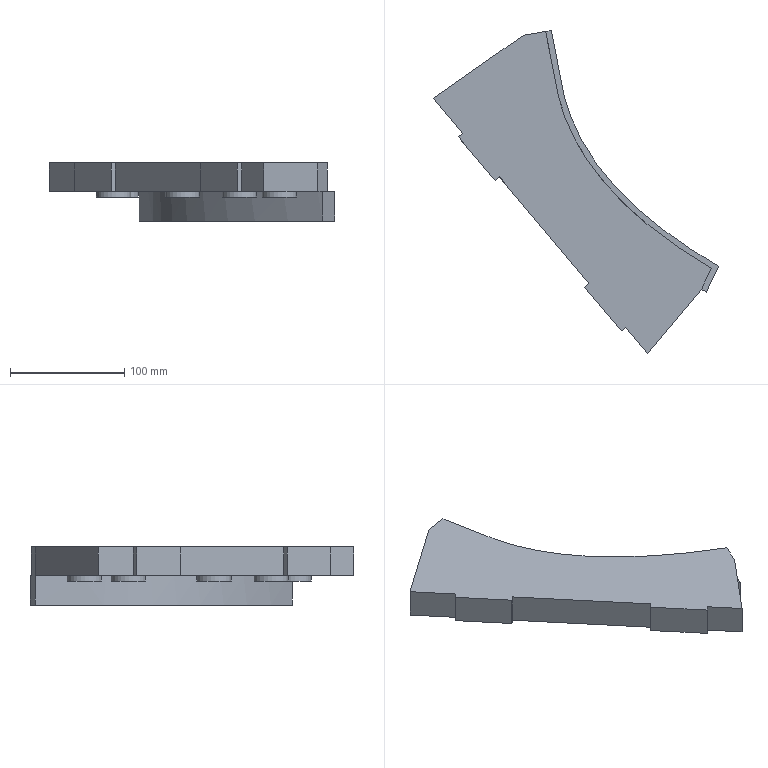Part | NX | features solid 2 | 1 solid | 31 faces | box 249.689 x 282.861 x 51 mm | volume 776005 mm3 | plane 23 | cylinder 5 | spline 3 | commonest cylinder face diameters 30 x5
STEP:
#1=CARTESIAN_POINT('',(-785.62,49.22,20.));
#2=VERTEX_POINT('',#1);
#3=CARTESIAN_POINT('',(-640.688,-158.312,20.));
#4=VERTEX_POINT('',#3);
#5=CARTESIAN_POINT('',(-785.62,49.22,20.));
#6=CARTESIAN_POINT('',(-784.592,43.889,20.));
#7=CARTESIAN_POINT('',(-782.539,33.228,20.));
#8=CARTESIAN_POINT('',(-779.967,19.892,20.));
#9=CARTESIAN_POINT('',(-777.921,9.245,20.));
#10=CARTESIAN_POINT('',(-776.403,1.242,20.));
#11=CARTESIAN_POINT('',(-774.716,-6.95,20.));
#12=CARTESIAN_POINT('',(-771.799,-17.805,20.));
#13=CARTESIAN_POINT('',(-767.13,-31.015,20.));
#14=CARTESIAN_POINT('',(-757.579,-51.275,20.));
#15=CARTESIAN_POINT('',(-742.261,-74.623,20.));
#16=CARTESIAN_POINT('',(-720.074,-99.485,20.));
#17=CARTESIAN_POINT('',(-687.034,-128.8,20.));
#18=CARTESIAN_POINT('',(-659.634,-147.246,20.));
#19=CARTESIAN_POINT('',(-640.688,-158.312,20.));
#20=B_SPLINE_CURVE_WITH_KNOTS('',3,(#5,#6,#7,#8,#9,#10,#11,#12,#13,#14,#15,#16,#17,#18,#19),.UNSPECIFIED.,.F.,.F.,(4,1,1,1,1,1,1,1,1,1,1,1,4),(-0.0002983,0.06115,0.1226,0.1533,0.184,0.2148,0.2455,0.3069,0.3684,0.4913,0.6141,0.737,0.9828),.UNSPECIFIED.);
#21=EDGE_CURVE('',#2,#4,#20,.T.);
#22=ORIENTED_EDGE('',*,*,#21,.T.);
#23=CARTESIAN_POINT('',(-649.178,-176.519,20.));
#24=VERTEX_POINT('',#23);
#25=CARTESIAN_POINT('',(-638.752,-154.162,20.));
#26=DIRECTION('',(-0.4226,-0.9063,0.));
#27=VECTOR('',#26,1000.);
#28=LINE('',#25,#27);
#29=EDGE_CURVE('',#4,#24,#28,.T.);
#30=ORIENTED_EDGE('',*,*,#29,.T.);
#31=CARTESIAN_POINT('',(-644.823,-179.011,20.));
#32=VERTEX_POINT('',#31);
#33=CARTESIAN_POINT('',(-805.318,45.747,20.));
#34=CARTESIAN_POINT('',(-803.55,36.568,20.));
#35=CARTESIAN_POINT('',(-801.348,25.134,20.));
#36=CARTESIAN_POINT('',(-798.703,11.417,20.));
#37=CARTESIAN_POINT('',(-797.422,4.72,20.));
#38=CARTESIAN_POINT('',(-796.1,-2.196,20.));
#39=CARTESIAN_POINT('',(-794.091,-12.171,20.));
#40=CARTESIAN_POINT('',(-790.472,-25.289,20.));
#41=CARTESIAN_POINT('',(-782.995,-45.31,20.));
#42=CARTESIAN_POINT('',(-770.656,-68.68,20.));
#43=CARTESIAN_POINT('',(-752.344,-93.703,20.));
#44=CARTESIAN_POINT('',(-731.663,-115.921,20.));
#45=CARTESIAN_POINT('',(-709.317,-135.702,20.));
#46=CARTESIAN_POINT('',(-680.689,-157.352,20.));
#47=CARTESIAN_POINT('',(-658.817,-171.096,20.));
#48=CARTESIAN_POINT('',(-644.823,-179.011,20.));
#49=B_SPLINE_CURVE_WITH_KNOTS('',3,(#33,#34,#35,#36,#37,#38,#39,#40,#41,#42,#43,#44,#45,#46,#47,#48),.UNSPECIFIED.,.F.,.F.,(4,1,1,1,1,1,1,1,1,1,1,1,1,4),(0.,0.1048,0.1307,0.1565,0.1824,0.2082,0.2599,0.3116,0.4149,0.5183,0.6217,0.725,0.8284,1.),.UNSPECIFIED.);
#50=EDGE_CURVE('',#32,#24,#49,.F.);
#51=ORIENTED_EDGE('',*,*,#50,.F.);
#52=CARTESIAN_POINT('',(-634.221,-156.275,20.));
#53=VERTEX_POINT('',#52);
#54=CARTESIAN_POINT('',(-634.221,-156.275,20.));
#55=DIRECTION('',(0.4226,0.9063,0.));
#56=VECTOR('',#55,1000.);
#57=LINE('',#54,#56);
#58=EDGE_CURVE('',#32,#53,#57,.T.);
#59=ORIENTED_EDGE('',*,*,#58,.T.);
#60=CARTESIAN_POINT('',(-780.695,50.088,20.));
#61=VERTEX_POINT('',#60);
#62=CARTESIAN_POINT('',(-780.695,50.088,20.));
#63=CARTESIAN_POINT('',(-778.803,40.269,20.));
#64=CARTESIAN_POINT('',(-776.28,27.176,20.));
#65=CARTESIAN_POINT('',(-773.127,10.811,20.));
#66=CARTESIAN_POINT('',(-771.556,2.503,20.));
#67=CARTESIAN_POINT('',(-770.053,-4.764,20.));
#68=CARTESIAN_POINT('',(-768.05,-12.691,20.));
#69=CARTESIAN_POINT('',(-763.621,-26.574,20.));
#70=CARTESIAN_POINT('',(-751.782,-52.713,20.));
#71=CARTESIAN_POINT('',(-727.402,-85.879,20.));
#72=CARTESIAN_POINT('',(-691.163,-119.147,20.));
#73=CARTESIAN_POINT('',(-659.144,-141.522,20.));
#74=CARTESIAN_POINT('',(-639.695,-153.145,20.));
#75=CARTESIAN_POINT('',(-634.221,-156.275,20.));
#76=B_SPLINE_CURVE_WITH_KNOTS('',3,(#62,#63,#64,#65,#66,#67,#68,#69,#70,#71,#72,#73,#74,#75),.UNSPECIFIED.,.F.,.F.,(4,1,1,1,1,1,1,1,1,1,1,4),(0.,0.1132,0.1509,0.1886,0.2088,0.2349,0.2811,0.3736,0.5586,0.7436,0.9286,1.),.UNSPECIFIED.);
#77=EDGE_CURVE('',#53,#61,#76,.F.);
#78=ORIENTED_EDGE('',*,*,#77,.T.);
#79=CARTESIAN_POINT('',(-780.695,50.088,20.));
#80=DIRECTION('',(0.9848,0.1736,0.));
#81=VECTOR('',#80,1000.);
#82=LINE('',#79,#81);
#83=EDGE_CURVE('',#2,#61,#82,.T.);
#84=ORIENTED_EDGE('',*,*,#83,.F.);
#85=EDGE_LOOP('',(#22,#30,#51,#59,#78,#84));
#86=FACE_BOUND('',#85,.T.);
#87=CARTESIAN_POINT('',(-565.659,-207.42,20.));
#88=DIRECTION('',(0.,0.,1.));
#89=DIRECTION('',(1.,0.,0.));
#90=AXIS2_PLACEMENT_3D('',#87,#88,#89);
#91=PLANE('',#90);
#92=ADVANCED_FACE('',(#86),#91,.T.);
#93=CARTESIAN_POINT('',(-669.708,-173.137,15.));
#94=VERTEX_POINT('',#93);
#95=CARTESIAN_POINT('',(-682.698,-180.637,15.));
#96=DIRECTION('',(0.,0.,-1.));
#97=DIRECTION('',(0.866,0.5,0.));
#98=AXIS2_PLACEMENT_3D('',#95,#96,#97);
#99=CIRCLE('',#98,15.);
#100=EDGE_CURVE('',#94,#94,#99,.T.);
#101=ORIENTED_EDGE('',*,*,#100,.T.);
#102=EDGE_LOOP('',(#101));
#103=FACE_BOUND('',#102,.T.);
#104=CARTESIAN_POINT('',(-682.698,-180.637,15.));
#105=DIRECTION('',(0.,0.,-1.));
#106=DIRECTION('',(-0.866,-0.5,0.));
#107=AXIS2_PLACEMENT_3D('',#104,#105,#106);
#108=PLANE('',#107);
#109=ADVANCED_FACE('',(#103),#108,.T.);
#110=ORIENTED_EDGE('',*,*,#100,.F.);
#111=EDGE_LOOP('',(#110));
#112=FACE_BOUND('',#111,.T.);
#113=CARTESIAN_POINT('',(-669.708,-173.137,20.));
#114=VERTEX_POINT('',#113);
#115=CARTESIAN_POINT('',(-682.698,-180.637,20.));
#116=DIRECTION('',(0.,0.,-1.));
#117=DIRECTION('',(0.866,0.5,0.));
#118=AXIS2_PLACEMENT_3D('',#115,#116,#117);
#119=CIRCLE('',#118,15.);
#120=EDGE_CURVE('',#114,#114,#119,.T.);
#121=ORIENTED_EDGE('',*,*,#120,.T.);
#122=EDGE_LOOP('',(#121));
#123=FACE_BOUND('',#122,.T.);
#124=CARTESIAN_POINT('',(-682.698,-180.637,20.));
#125=DIRECTION('',(0.,0.,-1.));
#126=DIRECTION('',(-0.866,-0.5,0.));
#127=AXIS2_PLACEMENT_3D('',#124,#125,#126);
#128=CYLINDRICAL_SURFACE('',#127,15.);
#129=ADVANCED_FACE('',(#112,#123),#128,.T.);
#130=CARTESIAN_POINT('',(-805.318,45.747,20.));
#131=VERTEX_POINT('',#130);
#132=CARTESIAN_POINT('',(-649.178,-176.519,20.));
#133=CARTESIAN_POINT('',(-659.441,-170.582,20.));
#134=CARTESIAN_POINT('',(-679.515,-158.013,20.));
#135=CARTESIAN_POINT('',(-708.226,-136.801,20.));
#136=CARTESIAN_POINT('',(-730.28,-117.148,20.));
#137=CARTESIAN_POINT('',(-746.505,-99.916,20.));
#138=CARTESIAN_POINT('',(-757.891,-86.111,20.));
#139=CARTESIAN_POINT('',(-768.135,-71.661,20.));
#140=CARTESIAN_POINT('',(-777.154,-56.472,20.));
#141=CARTESIAN_POINT('',(-784.851,-40.491,20.));
#142=CARTESIAN_POINT('',(-790.016,-26.444,20.));
#143=CARTESIAN_POINT('',(-793.291,-15.081,20.));
#144=CARTESIAN_POINT('',(-795.289,-6.451,20.));
#145=CARTESIAN_POINT('',(-796.948,2.251,20.));
#146=CARTESIAN_POINT('',(-799.169,13.852,20.));
#147=CARTESIAN_POINT('',(-801.968,28.349,20.));
#148=CARTESIAN_POINT('',(-804.201,39.947,20.));
#149=CARTESIAN_POINT('',(-805.318,45.747,20.));
#150=B_SPLINE_CURVE_WITH_KNOTS('',3,(#132,#133,#134,#135,#136,#137,#138,#139,#140,#141,#142,#143,#144,#145,#146,#147,#148,#149),.UNSPECIFIED.,.F.,.F.,(4,1,1,1,1,1,1,1,1,1,1,1,1,1,1,4),(0.1002,0.1358,0.1714,0.207,0.2248,0.2425,0.2603,0.2781,0.2959,0.3137,0.3226,0.3315,0.3404,0.3493,0.3671,0.3849),.UNSPECIFIED.);
#151=EDGE_CURVE('',#131,#24,#150,.F.);
#152=ORIENTED_EDGE('',*,*,#151,.F.);
#153=CARTESIAN_POINT('',(-805.318,45.747,-6.));
#154=VERTEX_POINT('',#153);
#155=CARTESIAN_POINT('',(-805.318,45.747,45.));
#156=DIRECTION('',(0.,0.,-1.));
#157=VECTOR('',#156,1000.);
#158=LINE('',#155,#157);
#159=EDGE_CURVE('',#131,#154,#158,.T.);
#160=ORIENTED_EDGE('',*,*,#159,.T.);
#161=CARTESIAN_POINT('',(-644.823,-179.011,-6.));
#162=VERTEX_POINT('',#161);
#163=CARTESIAN_POINT('',(-805.318,45.747,-6.));
#164=CARTESIAN_POINT('',(-803.55,36.568,-6.));
#165=CARTESIAN_POINT('',(-801.348,25.134,-6.));
#166=CARTESIAN_POINT('',(-798.703,11.417,-6.));
#167=CARTESIAN_POINT('',(-797.422,4.72,-6.));
#168=CARTESIAN_POINT('',(-796.1,-2.196,-6.));
#169=CARTESIAN_POINT('',(-794.091,-12.171,-6.));
#170=CARTESIAN_POINT('',(-790.472,-25.289,-6.));
#171=CARTESIAN_POINT('',(-782.995,-45.31,-6.));
#172=CARTESIAN_POINT('',(-770.656,-68.68,-6.));
#173=CARTESIAN_POINT('',(-752.344,-93.703,-6.));
#174=CARTESIAN_POINT('',(-731.663,-115.921,-6.));
#175=CARTESIAN_POINT('',(-709.317,-135.702,-6.));
#176=CARTESIAN_POINT('',(-680.689,-157.352,-6.));
#177=CARTESIAN_POINT('',(-658.817,-171.096,-6.));
#178=CARTESIAN_POINT('',(-644.823,-179.011,-6.));
#179=B_SPLINE_CURVE_WITH_KNOTS('',3,(#163,#164,#165,#166,#167,#168,#169,#170,#171,#172,#173,#174,#175,#176,#177,#178),.UNSPECIFIED.,.F.,.F.,(4,1,1,1,1,1,1,1,1,1,1,1,1,4),(0.,0.1048,0.1307,0.1565,0.1824,0.2082,0.2599,0.3116,0.4149,0.5183,0.6217,0.725,0.8284,1.),.UNSPECIFIED.);
#180=EDGE_CURVE('',#154,#162,#179,.T.);
#181=ORIENTED_EDGE('',*,*,#180,.T.);
#182=CARTESIAN_POINT('',(-644.823,-179.011,45.));
#183=DIRECTION('',(0.,0.,-1.));
#184=VECTOR('',#183,1000.);
#185=LINE('',#182,#184);
#186=EDGE_CURVE('',#32,#162,#185,.T.);
#187=ORIENTED_EDGE('',*,*,#186,.F.);
#188=ORIENTED_EDGE('',*,*,#50,.T.);
#189=EDGE_LOOP('',(#152,#160,#181,#187,#188));
#190=FACE_BOUND('',#189,.T.);
#191=CARTESIAN_POINT('',(-805.318,45.747,20.));
#192=CARTESIAN_POINT('',(-805.318,45.747,-6.));
#193=CARTESIAN_POINT('',(-804.264,40.275,20.));
#194=CARTESIAN_POINT('',(-804.264,40.275,-6.));
#195=CARTESIAN_POINT('',(-802.161,29.355,20.));
#196=CARTESIAN_POINT('',(-802.161,29.355,-6.));
#197=CARTESIAN_POINT('',(-799.507,15.599,20.));
#198=CARTESIAN_POINT('',(-799.507,15.599,-6.));
#199=CARTESIAN_POINT('',(-797.435,4.808,20.));
#200=CARTESIAN_POINT('',(-797.435,4.808,-6.));
#201=CARTESIAN_POINT('',(-795.845,-3.597,20.));
#202=CARTESIAN_POINT('',(-795.845,-3.597,-6.));
#203=CARTESIAN_POINT('',(-793.889,-12.805,20.));
#204=CARTESIAN_POINT('',(-793.889,-12.805,-6.));
#205=CARTESIAN_POINT('',(-790.396,-25.393,20.));
#206=CARTESIAN_POINT('',(-790.396,-25.393,-6.));
#207=CARTESIAN_POINT('',(-784.843,-40.631,20.));
#208=CARTESIAN_POINT('',(-784.843,-40.631,-6.));
#209=CARTESIAN_POINT('',(-776.44,-57.876,20.));
#210=CARTESIAN_POINT('',(-776.44,-57.876,-6.));
#211=CARTESIAN_POINT('',(-766.575,-74.079,20.));
#212=CARTESIAN_POINT('',(-766.575,-74.079,-6.));
#213=CARTESIAN_POINT('',(-751.833,-94.216,20.));
#214=CARTESIAN_POINT('',(-751.833,-94.216,-6.));
#215=CARTESIAN_POINT('',(-731.088,-116.783,20.));
#216=CARTESIAN_POINT('',(-731.088,-116.783,-6.));
#217=CARTESIAN_POINT('',(-703.818,-140.307,20.));
#218=CARTESIAN_POINT('',(-703.818,-140.307,-6.));
#219=CARTESIAN_POINT('',(-675.037,-161.006,20.));
#220=CARTESIAN_POINT('',(-675.037,-161.006,-6.));
#221=CARTESIAN_POINT('',(-655.017,-173.245,20.));
#222=CARTESIAN_POINT('',(-655.017,-173.245,-6.));
#223=CARTESIAN_POINT('',(-644.823,-179.011,20.));
#224=CARTESIAN_POINT('',(-644.823,-179.011,-6.));
#225=B_SPLINE_SURFACE_WITH_KNOTS('',3,1,((#191,#192),(#193,#194),(#195,#196),(#197,#198),(#199,#200),(#201,#202),(#203,#204),(#205,#206),(#207,#208),(#209,#210),(#211,#212),(#213,#214),(#215,#216),(#217,#218),(#219,#220),(#221,#222),(#223,#224)),.SURF_OF_LINEAR_EXTRUSION.,.F.,.F.,.F.,(4,1,1,1,1,1,1,1,1,1,1,1,1,1,4),(2,2),(0.,0.0625,0.125,0.1562,0.1875,0.2188,0.25,0.3125,0.375,0.4375,0.5,0.625,0.75,0.875,1.),(0.,1.),.UNSPECIFIED.);
#226=ADVANCED_FACE('',(#190),#225,.F.);
#227=CARTESIAN_POINT('',(-634.221,-156.275,-6.));
#228=VERTEX_POINT('',#227);
#229=CARTESIAN_POINT('',(-634.221,-156.275,-6.));
#230=DIRECTION('',(-0.4226,-0.9063,0.));
#231=VECTOR('',#230,1000.);
#232=LINE('',#229,#231);
#233=EDGE_CURVE('',#228,#162,#232,.T.);
#234=ORIENTED_EDGE('',*,*,#233,.F.);
#235=CARTESIAN_POINT('',(-634.221,-156.275,45.));
#236=DIRECTION('',(0.,0.,-1.));
#237=VECTOR('',#236,1000.);
#238=LINE('',#235,#237);
#239=EDGE_CURVE('',#53,#228,#238,.T.);
#240=ORIENTED_EDGE('',*,*,#239,.F.);
#241=ORIENTED_EDGE('',*,*,#58,.F.);
#242=ORIENTED_EDGE('',*,*,#186,.T.);
#243=EDGE_LOOP('',(#234,#240,#241,#242));
#244=FACE_BOUND('',#243,.T.);
#245=CARTESIAN_POINT('',(-644.823,-179.011,45.));
#246=DIRECTION('',(0.9063,-0.4226,0.));
#247=DIRECTION('',(0.4226,0.9063,0.));
#248=AXIS2_PLACEMENT_3D('',#245,#246,#247);
#249=PLANE('',#248);
#250=ADVANCED_FACE('',(#244),#249,.T.);
#251=CARTESIAN_POINT('',(-649.178,-176.519,45.));
#252=VERTEX_POINT('',#251);
#253=CARTESIAN_POINT('',(-649.178,-176.519,20.));
#254=DIRECTION('',(0.,0.,-1.));
#255=VECTOR('',#254,1000.);
#256=LINE('',#253,#255);
#257=EDGE_CURVE('',#252,#24,#256,.T.);
#258=ORIENTED_EDGE('',*,*,#257,.F.);
#259=CARTESIAN_POINT('',(-696.38,-232.773,45.));
#260=VERTEX_POINT('',#259);
#261=CARTESIAN_POINT('',(-649.96,-177.452,45.));
#262=DIRECTION('',(-0.6428,-0.766,0.));
#263=VECTOR('',#262,1000.);
#264=LINE('',#261,#263);
#265=EDGE_CURVE('',#252,#260,#264,.T.);
#266=ORIENTED_EDGE('',*,*,#265,.T.);
#267=CARTESIAN_POINT('',(-696.38,-232.773,20.));
#268=VERTEX_POINT('',#267);
#269=CARTESIAN_POINT('',(-696.38,-232.773,45.));
#270=DIRECTION('',(0.,0.,-1.));
#271=VECTOR('',#270,1000.);
#272=LINE('',#269,#271);
#273=EDGE_CURVE('',#260,#268,#272,.T.);
#274=ORIENTED_EDGE('',*,*,#273,.T.);
#275=CARTESIAN_POINT('',(-649.96,-177.452,20.));
#276=DIRECTION('',(-0.6428,-0.766,0.));
#277=VECTOR('',#276,1000.);
#278=LINE('',#275,#277);
#279=EDGE_CURVE('',#24,#268,#278,.T.);
#280=ORIENTED_EDGE('',*,*,#279,.F.);
#281=EDGE_LOOP('',(#258,#266,#274,#280));
#282=FACE_BOUND('',#281,.T.);
#283=CARTESIAN_POINT('',(-649.178,-176.519,20.));
#284=DIRECTION('',(-0.766,0.6428,0.));
#285=DIRECTION('',(-0.6428,-0.766,0.));
#286=AXIS2_PLACEMENT_3D('',#283,#284,#285);
#287=PLANE('',#286);
#288=ADVANCED_FACE('',(#282),#287,.F.);
#289=ORIENTED_EDGE('',*,*,#29,.F.);
#290=CARTESIAN_POINT('',(-640.688,-158.312,45.));
#291=VERTEX_POINT('',#290);
#292=CARTESIAN_POINT('',(-640.688,-158.312,32.5));
#293=DIRECTION('',(0.,0.,1.));
#294=VECTOR('',#293,1000.);
#295=LINE('',#292,#294);
#296=EDGE_CURVE('',#291,#4,#295,.F.);
#297=ORIENTED_EDGE('',*,*,#296,.F.);
#298=CARTESIAN_POINT('',(-634.625,-145.31,45.));
#299=DIRECTION('',(-0.4226,-0.9063,0.));
#300=VECTOR('',#299,1000.);
#301=LINE('',#298,#300);
#302=EDGE_CURVE('',#291,#252,#301,.T.);
#303=ORIENTED_EDGE('',*,*,#302,.T.);
#304=ORIENTED_EDGE('',*,*,#257,.T.);
#305=EDGE_LOOP('',(#289,#297,#303,#304));
#306=FACE_BOUND('',#305,.T.);
#307=CARTESIAN_POINT('',(-638.752,-154.162,20.));
#308=DIRECTION('',(-0.9063,0.4226,0.));
#309=DIRECTION('',(-0.4226,-0.9063,0.));
#310=AXIS2_PLACEMENT_3D('',#307,#308,#309);
#311=PLANE('',#310);
#312=ADVANCED_FACE('',(#306),#311,.F.);
#313=CARTESIAN_POINT('',(-715.664,-209.791,45.));
#314=VERTEX_POINT('',#313);
#315=CARTESIAN_POINT('',(-715.664,-209.791,20.));
#316=VERTEX_POINT('',#315);
#317=CARTESIAN_POINT('',(-715.664,-209.791,45.));
#318=DIRECTION('',(0.,0.,-1.));
#319=VECTOR('',#318,1000.);
#320=LINE('',#317,#319);
#321=EDGE_CURVE('',#314,#316,#320,.T.);
#322=ORIENTED_EDGE('',*,*,#321,.F.);
#323=CARTESIAN_POINT('',(-719.494,-213.005,45.));
#324=VERTEX_POINT('',#323);
#325=CARTESIAN_POINT('',(-719.494,-213.005,45.));
#326=DIRECTION('',(0.766,0.6428,0.));
#327=VECTOR('',#326,1000.);
#328=LINE('',#325,#327);
#329=EDGE_CURVE('',#324,#314,#328,.T.);
#330=ORIENTED_EDGE('',*,*,#329,.F.);
#331=CARTESIAN_POINT('',(-719.494,-213.005,20.));
#332=VERTEX_POINT('',#331);
#333=CARTESIAN_POINT('',(-719.494,-213.005,45.));
#334=DIRECTION('',(0.,0.,-1.));
#335=VECTOR('',#334,1000.);
#336=LINE('',#333,#335);
#337=EDGE_CURVE('',#324,#332,#336,.T.);
#338=ORIENTED_EDGE('',*,*,#337,.T.);
#339=CARTESIAN_POINT('',(-719.494,-213.005,20.));
#340=DIRECTION('',(0.766,0.6428,0.));
#341=VECTOR('',#340,1000.);
#342=LINE('',#339,#341);
#343=EDGE_CURVE('',#332,#316,#342,.T.);
#344=ORIENTED_EDGE('',*,*,#343,.T.);
#345=EDGE_LOOP('',(#322,#330,#338,#344));
#346=FACE_BOUND('',#345,.T.);
#347=CARTESIAN_POINT('',(-719.494,-213.005,45.));
#348=DIRECTION('',(0.6428,-0.766,0.));
#349=DIRECTION('',(0.766,0.6428,0.));
#350=AXIS2_PLACEMENT_3D('',#347,#348,#349);
#351=PLANE('',#350);
#352=ADVANCED_FACE('',(#346),#351,.T.);
#353=ORIENTED_EDGE('',*,*,#321,.T.);
#354=CARTESIAN_POINT('',(-676.357,-256.636,20.));
#355=DIRECTION('',(-0.6428,0.766,0.));
#356=VECTOR('',#355,1000.);
#357=LINE('',#354,#356);
#358=EDGE_CURVE('',#268,#316,#357,.T.);
#359=ORIENTED_EDGE('',*,*,#358,.F.);
#360=ORIENTED_EDGE('',*,*,#273,.F.);
#361=CARTESIAN_POINT('',(-676.357,-256.636,45.));
#362=DIRECTION('',(-0.6428,0.766,0.));
#363=VECTOR('',#362,1000.);
#364=LINE('',#361,#363);
#365=EDGE_CURVE('',#260,#314,#364,.T.);
#366=ORIENTED_EDGE('',*,*,#365,.T.);
#367=EDGE_LOOP('',(#353,#359,#360,#366));
#368=FACE_BOUND('',#367,.T.);
#369=CARTESIAN_POINT('',(-676.357,-256.636,45.));
#370=DIRECTION('',(-0.766,-0.6428,0.));
#371=DIRECTION('',(0.6428,-0.766,0.));
#372=AXIS2_PLACEMENT_3D('',#369,#370,#371);
#373=PLANE('',#372);
#374=ADVANCED_FACE('',(#368),#373,.T.);
#375=CARTESIAN_POINT('',(-862.028,-43.139,45.));
#376=VERTEX_POINT('',#375);
#377=CARTESIAN_POINT('',(-858.198,-39.926,45.));
#378=VERTEX_POINT('',#377);
#379=CARTESIAN_POINT('',(-1200.954,-327.532,45.));
#380=DIRECTION('',(0.766,0.6428,0.));
#381=VECTOR('',#380,1000.);
#382=LINE('',#379,#381);
#383=EDGE_CURVE('',#376,#378,#382,.T.);
#384=ORIENTED_EDGE('',*,*,#383,.F.);
#385=CARTESIAN_POINT('',(-829.889,-81.442,45.));
#386=VERTEX_POINT('',#385);
#387=CARTESIAN_POINT('',(-816.294,-97.644,45.));
#388=DIRECTION('',(-0.6428,0.766,0.));
#389=VECTOR('',#388,1000.);
#390=LINE('',#387,#389);
#391=EDGE_CURVE('',#386,#376,#390,.T.);
#392=ORIENTED_EDGE('',*,*,#391,.F.);
#393=CARTESIAN_POINT('',(-826.059,-78.228,45.));
#394=VERTEX_POINT('',#393);
#395=CARTESIAN_POINT('',(-1168.815,-365.834,45.));
#396=DIRECTION('',(0.766,0.6428,0.));
#397=VECTOR('',#396,1000.);
#398=LINE('',#395,#397);
#399=EDGE_CURVE('',#386,#394,#398,.T.);
#400=ORIENTED_EDGE('',*,*,#399,.T.);
#401=CARTESIAN_POINT('',(-747.803,-171.489,45.));
#402=VERTEX_POINT('',#401);
#403=CARTESIAN_POINT('',(-676.357,-256.636,45.));
#404=DIRECTION('',(-0.6428,0.766,0.));
#405=VECTOR('',#404,1000.);
#406=LINE('',#403,#405);
#407=EDGE_CURVE('',#402,#394,#406,.T.);
#408=ORIENTED_EDGE('',*,*,#407,.F.);
#409=CARTESIAN_POINT('',(-751.633,-174.703,45.));
#410=VERTEX_POINT('',#409);
#411=CARTESIAN_POINT('',(-751.633,-174.703,45.));
#412=DIRECTION('',(0.766,0.6428,0.));
#413=VECTOR('',#412,1000.);
#414=LINE('',#411,#413);
#415=EDGE_CURVE('',#410,#402,#414,.T.);
#416=ORIENTED_EDGE('',*,*,#415,.F.);
#417=CARTESIAN_POINT('',(-680.187,-259.85,45.));
#418=DIRECTION('',(-0.6428,0.766,0.));
#419=VECTOR('',#418,1000.);
#420=LINE('',#417,#419);
#421=EDGE_CURVE('',#324,#410,#420,.T.);
#422=ORIENTED_EDGE('',*,*,#421,.F.);
#423=ORIENTED_EDGE('',*,*,#329,.T.);
#424=ORIENTED_EDGE('',*,*,#365,.F.);
#425=ORIENTED_EDGE('',*,*,#265,.F.);
#426=ORIENTED_EDGE('',*,*,#302,.F.);
#427=CARTESIAN_POINT('',(-785.62,49.22,45.));
#428=VERTEX_POINT('',#427);
#429=CARTESIAN_POINT('',(-640.688,-158.312,45.));
#430=CARTESIAN_POINT('',(-645.683,-155.395,45.));
#431=CARTESIAN_POINT('',(-655.437,-149.467,45.));
#432=CARTESIAN_POINT('',(-667.042,-141.829,45.));
#433=CARTESIAN_POINT('',(-675.972,-135.582,45.));
#434=CARTESIAN_POINT('',(-681.406,-131.619,45.));
#435=CARTESIAN_POINT('',(-685.664,-128.416,45.));
#436=CARTESIAN_POINT('',(-688.818,-125.992,45.));
#437=CARTESIAN_POINT('',(-691.393,-123.972,45.));
#438=CARTESIAN_POINT('',(-693.468,-122.317,45.));
#439=CARTESIAN_POINT('',(-694.913,-121.153,45.));
#440=CARTESIAN_POINT('',(-696.729,-119.673,45.));
#441=CARTESIAN_POINT('',(-698.99,-117.805,45.));
#442=CARTESIAN_POINT('',(-701.817,-115.425,45.));
#443=CARTESIAN_POINT('',(-705.118,-112.571,45.));
#444=CARTESIAN_POINT('',(-709.43,-108.744,45.));
#445=CARTESIAN_POINT('',(-714.638,-103.929,45.));
#446=CARTESIAN_POINT('',(-720.599,-98.098,45.));
#447=CARTESIAN_POINT('',(-726.271,-92.216,45.));
#448=CARTESIAN_POINT('',(-730.758,-87.27,45.));
#449=CARTESIAN_POINT('',(-734.202,-83.29,45.));
#450=CARTESIAN_POINT('',(-736.717,-80.286,45.));
#451=CARTESIAN_POINT('',(-738.739,-77.789,45.));
#452=CARTESIAN_POINT('',(-740.351,-75.747,45.));
#453=CARTESIAN_POINT('',(-741.461,-74.317,45.));
#454=CARTESIAN_POINT('',(-742.858,-72.483,45.));
#455=CARTESIAN_POINT('',(-744.58,-70.172,45.));
#456=CARTESIAN_POINT('',(-746.71,-67.224,45.));
#457=CARTESIAN_POINT('',(-749.153,-63.689,45.));
#458=CARTESIAN_POINT('',(-752.287,-58.945,45.));
#459=CARTESIAN_POINT('',(-755.961,-52.973,45.));
#460=CARTESIAN_POINT('',(-761.328,-43.322,45.));
#461=CARTESIAN_POINT('',(-765.921,-33.534,45.));
#462=CARTESIAN_POINT('',(-769.268,-24.835,45.));
#463=CARTESIAN_POINT('',(-770.769,-20.468,45.));
#464=CARTESIAN_POINT('',(-771.584,-17.943,45.));
#465=CARTESIAN_POINT('',(-772.155,-16.103,45.));
#466=CARTESIAN_POINT('',(-772.767,-14.036,45.));
#467=CARTESIAN_POINT('',(-773.329,-12.038,45.));
#468=CARTESIAN_POINT('',(-773.78,-10.353,45.));
#469=CARTESIAN_POINT('',(-774.119,-9.032,45.));
#470=CARTESIAN_POINT('',(-774.382,-7.979,45.));
#471=CARTESIAN_POINT('',(-774.578,-7.17,45.));
#472=CARTESIAN_POINT('',(-774.869,-5.935,45.));
#473=CARTESIAN_POINT('',(-775.232,-4.321,45.));
#474=CARTESIAN_POINT('',(-775.612,-2.548,45.));
#475=CARTESIAN_POINT('',(-775.881,-1.246,45.));
#476=CARTESIAN_POINT('',(-776.02,-0.5615,45.));
#477=CARTESIAN_POINT('',(-776.096,-0.1885,45.));
#478=CARTESIAN_POINT('',(-776.165,0.1598,45.));
#479=CARTESIAN_POINT('',(-776.185,0.2589,45.));
#480=CARTESIAN_POINT('',(-776.231,0.4876,45.));
#481=CARTESIAN_POINT('',(-776.306,0.8667,45.));
#482=CARTESIAN_POINT('',(-776.429,1.488,45.));
#483=CARTESIAN_POINT('',(-776.591,2.317,45.));
#484=CARTESIAN_POINT('',(-776.831,3.549,45.));
#485=CARTESIAN_POINT('',(-777.105,4.966,45.));
#486=CARTESIAN_POINT('',(-777.412,6.566,45.));
#487=CARTESIAN_POINT('',(-777.62,7.65,45.));
#488=CARTESIAN_POINT('',(-777.791,8.546,45.));
#489=CARTESIAN_POINT('',(-777.91,9.167,45.));
#490=CARTESIAN_POINT('',(-777.988,9.581,45.));
#491=CARTESIAN_POINT('',(-778.038,9.839,45.));
#492=CARTESIAN_POINT('',(-778.14,10.375,45.));
#493=CARTESIAN_POINT('',(-778.285,11.133,45.));
#494=CARTESIAN_POINT('',(-778.472,12.107,45.));
#495=CARTESIAN_POINT('',(-778.667,13.126,45.));
#496=CARTESIAN_POINT('',(-778.838,14.016,45.));
#497=CARTESIAN_POINT('',(-778.98,14.754,45.));
#498=CARTESIAN_POINT('',(-779.087,15.313,45.));
#499=CARTESIAN_POINT('',(-779.183,15.81,45.));
#500=CARTESIAN_POINT('',(-779.251,16.168,45.));
#501=CARTESIAN_POINT('',(-779.328,16.565,45.));
#502=CARTESIAN_POINT('',(-779.312,16.482,45.));
#503=CARTESIAN_POINT('',(-779.324,16.545,45.));
#504=CARTESIAN_POINT('',(-779.33,16.575,45.));
#505=CARTESIAN_POINT('',(-779.345,16.651,45.));
#506=CARTESIAN_POINT('',(-779.366,16.763,45.));
#507=CARTESIAN_POINT('',(-779.401,16.944,45.));
#508=CARTESIAN_POINT('',(-779.472,17.312,45.));
#509=CARTESIAN_POINT('',(-779.589,17.921,45.));
#510=CARTESIAN_POINT('',(-779.776,18.891,45.));
#511=CARTESIAN_POINT('',(-780.009,20.1,45.));
#512=CARTESIAN_POINT('',(-780.381,22.031,45.));
#513=CARTESIAN_POINT('',(-780.961,25.042,45.));
#514=CARTESIAN_POINT('',(-781.842,29.612,45.));
#515=CARTESIAN_POINT('',(-783.261,36.981,45.));
#516=CARTESIAN_POINT('',(-784.603,43.942,45.));
#517=CARTESIAN_POINT('',(-785.62,49.22,45.));
#518=B_SPLINE_CURVE_WITH_KNOTS('',3,(#429,#430,#431,#432,#433,#434,#435,#436,#437,#438,#439,#440,#441,#442,#443,#444,#445,#446,#447,#448,#449,#450,#451,#452,#453,#454,#455,#456,#457,#458,#459,#460,#461,#462,#463,#464,#465,#466,#467,#468,#469,#470,#471,#472,#473,#474,#475,#476,#477,#478,#479,#480,#481,#482,#483,#484,#485,#486,#487,#488,#489,#490,#491,#492,#493,#494,#495,#496,#497,#498,#499,#500,#501,#502,#503,#504,#505,#506,#507,#508,#509,#510,#511,#512,#513,#514,#515,#516,#517),.UNSPECIFIED.,.F.,.F.,(4,1,1,1,1,1,1,1,1,1,1,1,1,1,1,1,1,1,1,1,1,1,1,1,1,1,1,1,1,1,1,1,1,1,1,1,1,1,1,1,1,1,1,1,1,1,1,1,1,1,1,1,1,1,1,1,1,1,1,1,1,1,1,1,1,1,1,1,1,1,1,1,1,1,1,1,1,1,1,1,1,1,1,1,1,1,4),(0.,0.0625,0.125,0.1562,0.1875,0.2031,0.2188,0.2344,0.2422,0.25,0.2578,0.2656,0.2812,0.2969,0.3125,0.3438,0.375,0.4062,0.4375,0.4531,0.4688,0.4844,0.4922,0.5,0.5078,0.5156,0.5312,0.5469,0.5625,0.5938,0.625,0.6875,0.7188,0.7344,0.7422,0.75,0.7578,0.7656,0.7734,0.7773,0.7812,0.7852,0.7891,0.7969,0.8047,0.8086,0.8105,0.8115,0.8125,0.8135,0.8145,0.8164,0.8203,0.8242,0.8281,0.8359,0.8398,0.8438,0.8457,0.8477,0.8486,0.8496,0.8516,0.8555,0.8594,0.8633,0.8672,0.8691,0.8711,0.873,0.874,0.875,0.876,0.877,0.8789,0.8809,0.8828,0.8867,0.8906,0.8984,0.9062,0.9141,0.9219,0.9375,0.9531,0.9688,1.),.UNSPECIFIED.);
#519=EDGE_CURVE('',#428,#291,#518,.F.);
#520=ORIENTED_EDGE('',*,*,#519,.F.);
#521=CARTESIAN_POINT('',(-805.318,45.747,45.));
#522=VERTEX_POINT('',#521);
#523=CARTESIAN_POINT('',(-805.318,45.747,45.));
#524=DIRECTION('',(-0.9848,-0.1736,0.));
#525=VECTOR('',#524,1000.);
#526=LINE('',#523,#525);
#527=EDGE_CURVE('',#428,#522,#526,.T.);
#528=ORIENTED_EDGE('',*,*,#527,.T.);
#529=CARTESIAN_POINT('',(-883.91,-9.284,45.));
#530=VERTEX_POINT('',#529);
#531=CARTESIAN_POINT('',(-835.112,24.885,45.));
#532=DIRECTION('',(-0.8192,-0.5736,0.));
#533=VECTOR('',#532,1000.);
#534=LINE('',#531,#533);
#535=EDGE_CURVE('',#522,#530,#534,.T.);
#536=ORIENTED_EDGE('',*,*,#535,.T.);
#537=CARTESIAN_POINT('',(-676.357,-256.636,45.));
#538=DIRECTION('',(-0.6428,0.766,0.));
#539=VECTOR('',#538,1000.);
#540=LINE('',#537,#539);
#541=EDGE_CURVE('',#378,#530,#540,.T.);
#542=ORIENTED_EDGE('',*,*,#541,.F.);
#543=EDGE_LOOP('',(#384,#392,#400,#408,#416,#422,#423,#424,#425,#426,#520,#528,#536,#542));
#544=FACE_BOUND('',#543,.T.);
#545=CARTESIAN_POINT('',(-918.37,-664.302,45.));
#546=DIRECTION('',(0.,0.,1.));
#547=DIRECTION('',(1.,0.,0.));
#548=AXIS2_PLACEMENT_3D('',#545,#546,#547);
#549=PLANE('',#548);
#550=ADVANCED_FACE('',(#544),#549,.T.);
#551=CARTESIAN_POINT('',(-814.708,-28.137,20.));
#552=VERTEX_POINT('',#551);
#553=CARTESIAN_POINT('',(-827.698,-35.637,20.));
#554=DIRECTION('',(0.,0.,-1.));
#555=DIRECTION('',(0.866,0.5,0.));
#556=AXIS2_PLACEMENT_3D('',#553,#554,#555);
#557=CIRCLE('',#556,15.);
#558=EDGE_CURVE('',#552,#552,#557,.T.);
#559=ORIENTED_EDGE('',*,*,#558,.F.);
#560=EDGE_LOOP('',(#559));
#561=FACE_BOUND('',#560,.T.);
#562=CARTESIAN_POINT('',(-751.633,-174.703,20.));
#563=VERTEX_POINT('',#562);
#564=CARTESIAN_POINT('',(-680.187,-259.85,20.));
#565=DIRECTION('',(-0.6428,0.766,0.));
#566=VECTOR('',#565,1000.);
#567=LINE('',#564,#566);
#568=EDGE_CURVE('',#332,#563,#567,.T.);
#569=ORIENTED_EDGE('',*,*,#568,.T.);
#570=CARTESIAN_POINT('',(-747.803,-171.489,20.));
#571=VERTEX_POINT('',#570);
#572=CARTESIAN_POINT('',(-751.633,-174.703,20.));
#573=DIRECTION('',(0.766,0.6428,0.));
#574=VECTOR('',#573,1000.);
#575=LINE('',#572,#574);
#576=EDGE_CURVE('',#563,#571,#575,.T.);
#577=ORIENTED_EDGE('',*,*,#576,.T.);
#578=CARTESIAN_POINT('',(-826.059,-78.228,20.));
#579=VERTEX_POINT('',#578);
#580=CARTESIAN_POINT('',(-676.357,-256.636,20.));
#581=DIRECTION('',(-0.6428,0.766,0.));
#582=VECTOR('',#581,1000.);
#583=LINE('',#580,#582);
#584=EDGE_CURVE('',#571,#579,#583,.T.);
#585=ORIENTED_EDGE('',*,*,#584,.T.);
#586=CARTESIAN_POINT('',(-829.889,-81.442,20.));
#587=VERTEX_POINT('',#586);
#588=CARTESIAN_POINT('',(-736.865,-3.385,20.));
#589=DIRECTION('',(-0.766,-0.6428,0.));
#590=VECTOR('',#589,1000.);
#591=LINE('',#588,#590);
#592=EDGE_CURVE('',#587,#579,#591,.F.);
#593=ORIENTED_EDGE('',*,*,#592,.F.);
#594=CARTESIAN_POINT('',(-862.028,-43.139,20.));
#595=VERTEX_POINT('',#594);
#596=CARTESIAN_POINT('',(-816.294,-97.644,20.));
#597=DIRECTION('',(-0.6428,0.766,0.));
#598=VECTOR('',#597,1000.);
#599=LINE('',#596,#598);
#600=EDGE_CURVE('',#587,#595,#599,.T.);
#601=ORIENTED_EDGE('',*,*,#600,.T.);
#602=CARTESIAN_POINT('',(-858.198,-39.926,20.));
#603=VERTEX_POINT('',#602);
#604=CARTESIAN_POINT('',(-769.004,34.917,20.));
#605=DIRECTION('',(-0.766,-0.6428,0.));
#606=VECTOR('',#605,1000.);
#607=LINE('',#604,#606);
#608=EDGE_CURVE('',#595,#603,#607,.F.);
#609=ORIENTED_EDGE('',*,*,#608,.T.);
#610=CARTESIAN_POINT('',(-883.91,-9.284,20.));
#611=VERTEX_POINT('',#610);
#612=CARTESIAN_POINT('',(-676.357,-256.636,20.));
#613=DIRECTION('',(-0.6428,0.766,0.));
#614=VECTOR('',#613,1000.);
#615=LINE('',#612,#614);
#616=EDGE_CURVE('',#603,#611,#615,.T.);
#617=ORIENTED_EDGE('',*,*,#616,.T.);
#618=CARTESIAN_POINT('',(-835.112,24.885,20.));
#619=DIRECTION('',(-0.8192,-0.5736,0.));
#620=VECTOR('',#619,1000.);
#621=LINE('',#618,#620);
#622=EDGE_CURVE('',#131,#611,#621,.T.);
#623=ORIENTED_EDGE('',*,*,#622,.F.);
#624=ORIENTED_EDGE('',*,*,#151,.T.);
#625=ORIENTED_EDGE('',*,*,#279,.T.);
#626=ORIENTED_EDGE('',*,*,#358,.T.);
#627=ORIENTED_EDGE('',*,*,#343,.F.);
#628=EDGE_LOOP('',(#569,#577,#585,#593,#601,#609,#617,#623,#624,#625,#626,#627));
#629=FACE_BOUND('',#628,.T.);
#630=CARTESIAN_POINT('',(-704.708,-153.137,20.));
#631=VERTEX_POINT('',#630);
#632=CARTESIAN_POINT('',(-717.698,-160.637,20.));
#633=DIRECTION('',(0.,0.,-1.));
#634=DIRECTION('',(0.866,0.5,0.));
#635=AXIS2_PLACEMENT_3D('',#632,#633,#634);
#636=CIRCLE('',#635,15.);
#637=EDGE_CURVE('',#631,#631,#636,.T.);
#638=ORIENTED_EDGE('',*,*,#637,.F.);
#639=EDGE_LOOP('',(#638));
#640=FACE_BOUND('',#639,.T.);
#641=CARTESIAN_POINT('',(-754.708,-103.137,20.));
#642=VERTEX_POINT('',#641);
#643=CARTESIAN_POINT('',(-767.698,-110.637,20.));
#644=DIRECTION('',(0.,0.,-1.));
#645=DIRECTION('',(0.866,0.5,0.));
#646=AXIS2_PLACEMENT_3D('',#643,#644,#645);
#647=CIRCLE('',#646,15.);
#648=EDGE_CURVE('',#642,#642,#647,.T.);
#649=ORIENTED_EDGE('',*,*,#648,.F.);
#650=EDGE_LOOP('',(#649));
#651=FACE_BOUND('',#650,.T.);
#652=ORIENTED_EDGE('',*,*,#120,.F.);
#653=EDGE_LOOP('',(#652));
#654=FACE_BOUND('',#653,.T.);
#655=CARTESIAN_POINT('',(-808.057,10.344,20.));
#656=VERTEX_POINT('',#655);
#657=CARTESIAN_POINT('',(-821.047,2.844,20.));
#658=DIRECTION('',(0.,0.,-1.));
#659=DIRECTION('',(0.866,0.5,0.));
#660=AXIS2_PLACEMENT_3D('',#657,#658,#659);
#661=CIRCLE('',#660,15.);
#662=EDGE_CURVE('',#656,#656,#661,.T.);
#663=ORIENTED_EDGE('',*,*,#662,.F.);
#664=EDGE_LOOP('',(#663));
#665=FACE_BOUND('',#664,.T.);
#666=CARTESIAN_POINT('',(-565.659,-207.42,20.));
#667=DIRECTION('',(0.,0.,-1.));
#668=DIRECTION('',(-1.,0.,0.));
#669=AXIS2_PLACEMENT_3D('',#666,#667,#668);
#670=PLANE('',#669);
#671=ADVANCED_FACE('',(#561,#629,#640,#651,#654,#665),#670,.T.);
#672=CARTESIAN_POINT('',(-754.708,-103.137,15.));
#673=VERTEX_POINT('',#672);
#674=CARTESIAN_POINT('',(-767.698,-110.637,15.));
#675=DIRECTION('',(0.,0.,-1.));
#676=DIRECTION('',(0.866,0.5,0.));
#677=AXIS2_PLACEMENT_3D('',#674,#675,#676);
#678=CIRCLE('',#677,15.);
#679=EDGE_CURVE('',#673,#673,#678,.T.);
#680=ORIENTED_EDGE('',*,*,#679,.T.);
#681=EDGE_LOOP('',(#680));
#682=FACE_BOUND('',#681,.T.);
#683=CARTESIAN_POINT('',(-785.611,-100.558,15.));
#684=DIRECTION('',(0.,0.,1.));
#685=DIRECTION('',(1.,0.,0.));
#686=AXIS2_PLACEMENT_3D('',#683,#684,#685);
#687=PLANE('',#686);
#688=ADVANCED_FACE('',(#682),#687,.F.);
#689=ORIENTED_EDGE('',*,*,#233,.T.);
#690=ORIENTED_EDGE('',*,*,#180,.F.);
#691=CARTESIAN_POINT('',(-780.695,50.088,-6.));
#692=VERTEX_POINT('',#691);
#693=CARTESIAN_POINT('',(-780.695,50.088,-6.));
#694=DIRECTION('',(-0.9848,-0.1736,0.));
#695=VECTOR('',#694,1000.);
#696=LINE('',#693,#695);
#697=EDGE_CURVE('',#692,#154,#696,.T.);
#698=ORIENTED_EDGE('',*,*,#697,.F.);
#699=CARTESIAN_POINT('',(-780.695,50.088,-6.));
#700=CARTESIAN_POINT('',(-778.803,40.269,-6.));
#701=CARTESIAN_POINT('',(-776.28,27.176,-6.));
#702=CARTESIAN_POINT('',(-773.127,10.811,-6.));
#703=CARTESIAN_POINT('',(-771.556,2.503,-6.));
#704=CARTESIAN_POINT('',(-770.053,-4.764,-6.));
#705=CARTESIAN_POINT('',(-768.05,-12.691,-6.));
#706=CARTESIAN_POINT('',(-763.621,-26.574,-6.));
#707=CARTESIAN_POINT('',(-751.782,-52.713,-6.));
#708=CARTESIAN_POINT('',(-727.402,-85.879,-6.));
#709=CARTESIAN_POINT('',(-691.163,-119.147,-6.));
#710=CARTESIAN_POINT('',(-659.144,-141.522,-6.));
#711=CARTESIAN_POINT('',(-639.695,-153.145,-6.));
#712=CARTESIAN_POINT('',(-634.221,-156.275,-6.));
#713=B_SPLINE_CURVE_WITH_KNOTS('',3,(#699,#700,#701,#702,#703,#704,#705,#706,#707,#708,#709,#710,#711,#712),.UNSPECIFIED.,.F.,.F.,(4,1,1,1,1,1,1,1,1,1,1,4),(0.,0.1132,0.1509,0.1886,0.2088,0.2349,0.2811,0.3736,0.5586,0.7436,0.9286,1.),.UNSPECIFIED.);
#714=EDGE_CURVE('',#692,#228,#713,.T.);
#715=ORIENTED_EDGE('',*,*,#714,.T.);
#716=EDGE_LOOP('',(#689,#690,#698,#715));
#717=FACE_BOUND('',#716,.T.);
#718=CARTESIAN_POINT('',(-918.37,-664.302,-6.));
#719=DIRECTION('',(0.,0.,1.));
#720=DIRECTION('',(1.,0.,0.));
#721=AXIS2_PLACEMENT_3D('',#718,#719,#720);
#722=PLANE('',#721);
#723=ADVANCED_FACE('',(#717),#722,.F.);
#724=ORIENTED_EDGE('',*,*,#519,.T.);
#725=ORIENTED_EDGE('',*,*,#296,.T.);
#726=ORIENTED_EDGE('',*,*,#21,.F.);
#727=CARTESIAN_POINT('',(-785.62,49.22,37.));
#728=DIRECTION('',(0.,0.,1.));
#729=VECTOR('',#728,1000.);
#730=LINE('',#727,#729);
#731=EDGE_CURVE('',#428,#2,#730,.F.);
#732=ORIENTED_EDGE('',*,*,#731,.F.);
#733=EDGE_LOOP('',(#724,#725,#726,#732));
#734=FACE_BOUND('',#733,.T.);
#735=CARTESIAN_POINT('',(-785.62,49.22,20.));
#736=CARTESIAN_POINT('',(-785.62,49.22,45.));
#737=CARTESIAN_POINT('',(-784.592,43.889,20.));
#738=CARTESIAN_POINT('',(-784.592,43.889,45.));
#739=CARTESIAN_POINT('',(-782.539,33.228,20.));
#740=CARTESIAN_POINT('',(-782.539,33.228,45.));
#741=CARTESIAN_POINT('',(-779.967,19.892,20.));
#742=CARTESIAN_POINT('',(-779.967,19.892,45.));
#743=CARTESIAN_POINT('',(-777.921,9.245,20.));
#744=CARTESIAN_POINT('',(-777.921,9.245,45.));
#745=CARTESIAN_POINT('',(-776.403,1.242,20.));
#746=CARTESIAN_POINT('',(-776.403,1.242,45.));
#747=CARTESIAN_POINT('',(-774.716,-6.95,20.));
#748=CARTESIAN_POINT('',(-774.716,-6.95,45.));
#749=CARTESIAN_POINT('',(-771.799,-17.805,20.));
#750=CARTESIAN_POINT('',(-771.799,-17.805,45.));
#751=CARTESIAN_POINT('',(-767.13,-31.015,20.));
#752=CARTESIAN_POINT('',(-767.13,-31.015,45.));
#753=CARTESIAN_POINT('',(-757.579,-51.275,20.));
#754=CARTESIAN_POINT('',(-757.579,-51.275,45.));
#755=CARTESIAN_POINT('',(-742.261,-74.623,20.));
#756=CARTESIAN_POINT('',(-742.261,-74.623,45.));
#757=CARTESIAN_POINT('',(-720.074,-99.485,20.));
#758=CARTESIAN_POINT('',(-720.074,-99.485,45.));
#759=CARTESIAN_POINT('',(-687.034,-128.8,20.));
#760=CARTESIAN_POINT('',(-687.034,-128.8,45.));
#761=CARTESIAN_POINT('',(-659.634,-147.246,20.));
#762=CARTESIAN_POINT('',(-659.634,-147.246,45.));
#763=CARTESIAN_POINT('',(-640.688,-158.312,20.));
#764=CARTESIAN_POINT('',(-640.688,-158.312,45.));
#765=B_SPLINE_SURFACE_WITH_KNOTS('',3,1,((#735,#736),(#737,#738),(#739,#740),(#741,#742),(#743,#744),(#745,#746),(#747,#748),(#749,#750),(#751,#752),(#753,#754),(#755,#756),(#757,#758),(#759,#760),(#761,#762),(#763,#764)),.SURF_OF_LINEAR_EXTRUSION.,.F.,.F.,.F.,(4,1,1,1,1,1,1,1,1,1,1,1,4),(2,2),(-0.0002983,0.06115,0.1226,0.1533,0.184,0.2148,0.2455,0.3069,0.3684,0.4913,0.6141,0.737,0.9828),(0.,1.),.UNSPECIFIED.);
#766=ADVANCED_FACE('',(#734),#765,.F.);
#767=ORIENTED_EDGE('',*,*,#714,.F.);
#768=CARTESIAN_POINT('',(-780.695,50.088,45.));
#769=DIRECTION('',(0.,0.,-1.));
#770=VECTOR('',#769,1000.);
#771=LINE('',#768,#770);
#772=EDGE_CURVE('',#61,#692,#771,.T.);
#773=ORIENTED_EDGE('',*,*,#772,.F.);
#774=ORIENTED_EDGE('',*,*,#77,.F.);
#775=ORIENTED_EDGE('',*,*,#239,.T.);
#776=EDGE_LOOP('',(#767,#773,#774,#775));
#777=FACE_BOUND('',#776,.T.);
#778=CARTESIAN_POINT('',(-780.695,50.088,20.));
#779=CARTESIAN_POINT('',(-780.695,50.088,-6.));
#780=CARTESIAN_POINT('',(-779.65,44.665,20.));
#781=CARTESIAN_POINT('',(-779.65,44.665,-6.));
#782=CARTESIAN_POINT('',(-777.561,33.819,20.));
#783=CARTESIAN_POINT('',(-777.561,33.819,-6.));
#784=CARTESIAN_POINT('',(-774.945,20.262,20.));
#785=CARTESIAN_POINT('',(-774.945,20.262,-6.));
#786=CARTESIAN_POINT('',(-772.864,9.414,20.));
#787=CARTESIAN_POINT('',(-772.864,9.414,-6.));
#788=CARTESIAN_POINT('',(-771.32,1.276,20.));
#789=CARTESIAN_POINT('',(-771.32,1.276,-6.));
#790=CARTESIAN_POINT('',(-769.602,-6.83,20.));
#791=CARTESIAN_POINT('',(-769.602,-6.83,-6.));
#792=CARTESIAN_POINT('',(-766.652,-17.481,20.));
#793=CARTESIAN_POINT('',(-766.652,-17.481,-6.));
#794=CARTESIAN_POINT('',(-761.937,-30.477,20.));
#795=CARTESIAN_POINT('',(-761.937,-30.477,-6.));
#796=CARTESIAN_POINT('',(-752.313,-50.393,20.));
#797=CARTESIAN_POINT('',(-752.313,-50.393,-6.));
#798=CARTESIAN_POINT('',(-736.881,-73.39,20.));
#799=CARTESIAN_POINT('',(-736.881,-73.39,-6.));
#800=CARTESIAN_POINT('',(-714.506,-97.952,20.));
#801=CARTESIAN_POINT('',(-714.506,-97.952,-6.));
#802=CARTESIAN_POINT('',(-681.129,-126.988,20.));
#803=CARTESIAN_POINT('',(-681.129,-126.988,-6.));
#804=CARTESIAN_POINT('',(-653.399,-145.312,20.));
#805=CARTESIAN_POINT('',(-653.399,-145.312,-6.));
#806=CARTESIAN_POINT('',(-634.221,-156.275,20.));
#807=CARTESIAN_POINT('',(-634.221,-156.275,-6.));
#808=B_SPLINE_SURFACE_WITH_KNOTS('',3,1,((#778,#779),(#780,#781),(#782,#783),(#784,#785),(#786,#787),(#788,#789),(#790,#791),(#792,#793),(#794,#795),(#796,#797),(#798,#799),(#800,#801),(#802,#803),(#804,#805),(#806,#807)),.SURF_OF_LINEAR_EXTRUSION.,.F.,.F.,.F.,(4,1,1,1,1,1,1,1,1,1,1,1,4),(2,2),(0.,0.0625,0.125,0.1562,0.1875,0.2188,0.25,0.3125,0.375,0.5,0.625,0.75,1.),(0.,1.),.UNSPECIFIED.);
#809=ADVANCED_FACE('',(#777),#808,.T.);
#810=ORIENTED_EDGE('',*,*,#648,.T.);
#811=EDGE_LOOP('',(#810));
#812=FACE_BOUND('',#811,.T.);
#813=ORIENTED_EDGE('',*,*,#679,.F.);
#814=EDGE_LOOP('',(#813));
#815=FACE_BOUND('',#814,.T.);
#816=CARTESIAN_POINT('',(-767.698,-110.637,20.));
#817=DIRECTION('',(0.,0.,-1.));
#818=DIRECTION('',(-0.866,-0.5,0.));
#819=AXIS2_PLACEMENT_3D('',#816,#817,#818);
#820=CYLINDRICAL_SURFACE('',#819,15.);
#821=ADVANCED_FACE('',(#812,#815),#820,.T.);
#822=CARTESIAN_POINT('',(-751.633,-174.703,45.));
#823=DIRECTION('',(0.,0.,-1.));
#824=VECTOR('',#823,1000.);
#825=LINE('',#822,#824);
#826=EDGE_CURVE('',#410,#563,#825,.T.);
#827=ORIENTED_EDGE('',*,*,#826,.T.);
#828=ORIENTED_EDGE('',*,*,#568,.F.);
#829=ORIENTED_EDGE('',*,*,#337,.F.);
#830=ORIENTED_EDGE('',*,*,#421,.T.);
#831=EDGE_LOOP('',(#827,#828,#829,#830));
#832=FACE_BOUND('',#831,.T.);
#833=CARTESIAN_POINT('',(-680.187,-259.85,45.));
#834=DIRECTION('',(-0.766,-0.6428,0.));
#835=DIRECTION('',(0.6428,-0.766,0.));
#836=AXIS2_PLACEMENT_3D('',#833,#834,#835);
#837=PLANE('',#836);
#838=ADVANCED_FACE('',(#832),#837,.T.);
#839=ORIENTED_EDGE('',*,*,#584,.F.);
#840=CARTESIAN_POINT('',(-747.803,-171.489,45.));
#841=DIRECTION('',(0.,0.,-1.));
#842=VECTOR('',#841,1000.);
#843=LINE('',#840,#842);
#844=EDGE_CURVE('',#402,#571,#843,.T.);
#845=ORIENTED_EDGE('',*,*,#844,.F.);
#846=ORIENTED_EDGE('',*,*,#407,.T.);
#847=CARTESIAN_POINT('',(-826.059,-78.228,45.));
#848=DIRECTION('',(0.,0.,-1.));
#849=VECTOR('',#848,1000.);
#850=LINE('',#847,#849);
#851=EDGE_CURVE('',#394,#579,#850,.T.);
#852=ORIENTED_EDGE('',*,*,#851,.T.);
#853=EDGE_LOOP('',(#839,#845,#846,#852));
#854=FACE_BOUND('',#853,.T.);
#855=CARTESIAN_POINT('',(-676.357,-256.636,45.));
#856=DIRECTION('',(-0.766,-0.6428,0.));
#857=DIRECTION('',(0.6428,-0.766,0.));
#858=AXIS2_PLACEMENT_3D('',#855,#856,#857);
#859=PLANE('',#858);
#860=ADVANCED_FACE('',(#854),#859,.T.);
#861=ORIENTED_EDGE('',*,*,#851,.F.);
#862=ORIENTED_EDGE('',*,*,#399,.F.);
#863=CARTESIAN_POINT('',(-829.889,-81.442,45.));
#864=DIRECTION('',(0.,0.,-1.));
#865=VECTOR('',#864,1000.);
#866=LINE('',#863,#865);
#867=EDGE_CURVE('',#386,#587,#866,.T.);
#868=ORIENTED_EDGE('',*,*,#867,.T.);
#869=ORIENTED_EDGE('',*,*,#592,.T.);
#870=EDGE_LOOP('',(#861,#862,#868,#869));
#871=FACE_BOUND('',#870,.T.);
#872=CARTESIAN_POINT('',(-829.889,-81.442,45.));
#873=DIRECTION('',(0.6428,-0.766,0.));
#874=DIRECTION('',(0.766,0.6428,0.));
#875=AXIS2_PLACEMENT_3D('',#872,#873,#874);
#876=PLANE('',#875);
#877=ADVANCED_FACE('',(#871),#876,.T.);
#878=ORIENTED_EDGE('',*,*,#391,.T.);
#879=CARTESIAN_POINT('',(-862.028,-43.139,45.));
#880=DIRECTION('',(0.,0.,-1.));
#881=VECTOR('',#880,1000.);
#882=LINE('',#879,#881);
#883=EDGE_CURVE('',#376,#595,#882,.T.);
#884=ORIENTED_EDGE('',*,*,#883,.T.);
#885=ORIENTED_EDGE('',*,*,#600,.F.);
#886=ORIENTED_EDGE('',*,*,#867,.F.);
#887=EDGE_LOOP('',(#878,#884,#885,#886));
#888=FACE_BOUND('',#887,.T.);
#889=CARTESIAN_POINT('',(-816.294,-97.644,45.));
#890=DIRECTION('',(-0.766,-0.6428,0.));
#891=DIRECTION('',(0.6428,-0.766,0.));
#892=AXIS2_PLACEMENT_3D('',#889,#890,#891);
#893=PLANE('',#892);
#894=ADVANCED_FACE('',(#888),#893,.T.);
#895=ORIENTED_EDGE('',*,*,#844,.T.);
#896=ORIENTED_EDGE('',*,*,#576,.F.);
#897=ORIENTED_EDGE('',*,*,#826,.F.);
#898=ORIENTED_EDGE('',*,*,#415,.T.);
#899=EDGE_LOOP('',(#895,#896,#897,#898));
#900=FACE_BOUND('',#899,.T.);
#901=CARTESIAN_POINT('',(-751.633,-174.703,45.));
#902=DIRECTION('',(0.6428,-0.766,0.));
#903=DIRECTION('',(0.766,0.6428,0.));
#904=AXIS2_PLACEMENT_3D('',#901,#902,#903);
#905=PLANE('',#904);
#906=ADVANCED_FACE('',(#900),#905,.F.);
#907=CARTESIAN_POINT('',(-858.198,-39.926,45.));
#908=DIRECTION('',(0.,0.,-1.));
#909=VECTOR('',#908,1000.);
#910=LINE('',#907,#909);
#911=EDGE_CURVE('',#378,#603,#910,.T.);
#912=ORIENTED_EDGE('',*,*,#911,.T.);
#913=ORIENTED_EDGE('',*,*,#608,.F.);
#914=ORIENTED_EDGE('',*,*,#883,.F.);
#915=ORIENTED_EDGE('',*,*,#383,.T.);
#916=EDGE_LOOP('',(#912,#913,#914,#915));
#917=FACE_BOUND('',#916,.T.);
#918=CARTESIAN_POINT('',(-862.028,-43.139,45.));
#919=DIRECTION('',(0.6428,-0.766,0.));
#920=DIRECTION('',(0.766,0.6428,0.));
#921=AXIS2_PLACEMENT_3D('',#918,#919,#920);
#922=PLANE('',#921);
#923=ADVANCED_FACE('',(#917),#922,.F.);
#924=CARTESIAN_POINT('',(-808.057,10.344,15.));
#925=VERTEX_POINT('',#924);
#926=CARTESIAN_POINT('',(-821.047,2.844,15.));
#927=DIRECTION('',(0.,0.,-1.));
#928=DIRECTION('',(0.866,0.5,0.));
#929=AXIS2_PLACEMENT_3D('',#926,#927,#928);
#930=CIRCLE('',#929,15.);
#931=EDGE_CURVE('',#925,#925,#930,.T.);
#932=ORIENTED_EDGE('',*,*,#931,.T.);
#933=EDGE_LOOP('',(#932));
#934=FACE_BOUND('',#933,.T.);
#935=CARTESIAN_POINT('',(-821.047,2.844,15.));
#936=DIRECTION('',(0.,0.,-1.));
#937=DIRECTION('',(-0.866,-0.5,0.));
#938=AXIS2_PLACEMENT_3D('',#935,#936,#937);
#939=PLANE('',#938);
#940=ADVANCED_FACE('',(#934),#939,.T.);
#941=ORIENTED_EDGE('',*,*,#662,.T.);
#942=EDGE_LOOP('',(#941));
#943=FACE_BOUND('',#942,.T.);
#944=ORIENTED_EDGE('',*,*,#931,.F.);
#945=EDGE_LOOP('',(#944));
#946=FACE_BOUND('',#945,.T.);
#947=CARTESIAN_POINT('',(-821.047,2.844,20.));
#948=DIRECTION('',(0.,0.,-1.));
#949=DIRECTION('',(-0.866,-0.5,0.));
#950=AXIS2_PLACEMENT_3D('',#947,#948,#949);
#951=CYLINDRICAL_SURFACE('',#950,15.);
#952=ADVANCED_FACE('',(#943,#946),#951,.T.);
#953=CARTESIAN_POINT('',(-814.708,-28.137,15.));
#954=VERTEX_POINT('',#953);
#955=CARTESIAN_POINT('',(-827.698,-35.637,15.));
#956=DIRECTION('',(0.,0.,-1.));
#957=DIRECTION('',(0.866,0.5,0.));
#958=AXIS2_PLACEMENT_3D('',#955,#956,#957);
#959=CIRCLE('',#958,15.);
#960=EDGE_CURVE('',#954,#954,#959,.T.);
#961=ORIENTED_EDGE('',*,*,#960,.T.);
#962=EDGE_LOOP('',(#961));
#963=FACE_BOUND('',#962,.T.);
#964=CARTESIAN_POINT('',(-827.698,-35.637,15.));
#965=DIRECTION('',(0.,0.,-1.));
#966=DIRECTION('',(-0.866,-0.5,0.));
#967=AXIS2_PLACEMENT_3D('',#964,#965,#966);
#968=PLANE('',#967);
#969=ADVANCED_FACE('',(#963),#968,.T.);
#970=ORIENTED_EDGE('',*,*,#558,.T.);
#971=EDGE_LOOP('',(#970));
#972=FACE_BOUND('',#971,.T.);
#973=ORIENTED_EDGE('',*,*,#960,.F.);
#974=EDGE_LOOP('',(#973));
#975=FACE_BOUND('',#974,.T.);
#976=CARTESIAN_POINT('',(-827.698,-35.637,20.));
#977=DIRECTION('',(0.,0.,-1.));
#978=DIRECTION('',(-0.866,-0.5,0.));
#979=AXIS2_PLACEMENT_3D('',#976,#977,#978);
#980=CYLINDRICAL_SURFACE('',#979,15.);
#981=ADVANCED_FACE('',(#972,#975),#980,.T.);
#982=ORIENTED_EDGE('',*,*,#535,.F.);
#983=CARTESIAN_POINT('',(-805.318,45.747,45.));
#984=DIRECTION('',(0.,0.,-1.));
#985=VECTOR('',#984,1000.);
#986=LINE('',#983,#985);
#987=EDGE_CURVE('',#522,#131,#986,.T.);
#988=ORIENTED_EDGE('',*,*,#987,.T.);
#989=ORIENTED_EDGE('',*,*,#622,.T.);
#990=CARTESIAN_POINT('',(-883.91,-9.284,45.));
#991=DIRECTION('',(0.,0.,-1.));
#992=VECTOR('',#991,1000.);
#993=LINE('',#990,#992);
#994=EDGE_CURVE('',#530,#611,#993,.T.);
#995=ORIENTED_EDGE('',*,*,#994,.F.);
#996=EDGE_LOOP('',(#982,#988,#989,#995));
#997=FACE_BOUND('',#996,.T.);
#998=CARTESIAN_POINT('',(-805.318,45.747,20.));
#999=DIRECTION('',(-0.5736,0.8192,0.));
#1000=DIRECTION('',(-0.8192,-0.5736,0.));
#1001=AXIS2_PLACEMENT_3D('',#998,#999,#1000);
#1002=PLANE('',#1001);
#1003=ADVANCED_FACE('',(#997),#1002,.T.);
#1004=ORIENTED_EDGE('',*,*,#987,.F.);
#1005=ORIENTED_EDGE('',*,*,#527,.F.);
#1006=ORIENTED_EDGE('',*,*,#731,.T.);
#1007=ORIENTED_EDGE('',*,*,#83,.T.);
#1008=ORIENTED_EDGE('',*,*,#772,.T.);
#1009=ORIENTED_EDGE('',*,*,#697,.T.);
#1010=ORIENTED_EDGE('',*,*,#159,.F.);
#1011=EDGE_LOOP('',(#1004,#1005,#1006,#1007,#1008,#1009,#1010));
#1012=FACE_BOUND('',#1011,.T.);
#1013=CARTESIAN_POINT('',(-805.318,45.747,45.));
#1014=DIRECTION('',(0.1736,-0.9848,0.));
#1015=DIRECTION('',(0.9848,0.1736,0.));
#1016=AXIS2_PLACEMENT_3D('',#1013,#1014,#1015);
#1017=PLANE('',#1016);
#1018=ADVANCED_FACE('',(#1012),#1017,.F.);
#1019=ORIENTED_EDGE('',*,*,#616,.F.);
#1020=ORIENTED_EDGE('',*,*,#911,.F.);
#1021=ORIENTED_EDGE('',*,*,#541,.T.);
#1022=ORIENTED_EDGE('',*,*,#994,.T.);
#1023=EDGE_LOOP('',(#1019,#1020,#1021,#1022));
#1024=FACE_BOUND('',#1023,.T.);
#1025=CARTESIAN_POINT('',(-676.357,-256.636,45.));
#1026=DIRECTION('',(-0.766,-0.6428,0.));
#1027=DIRECTION('',(0.6428,-0.766,0.));
#1028=AXIS2_PLACEMENT_3D('',#1025,#1026,#1027);
#1029=PLANE('',#1028);
#1030=ADVANCED_FACE('',(#1024),#1029,.T.);
#1031=ORIENTED_EDGE('',*,*,#637,.T.);
#1032=EDGE_LOOP('',(#1031));
#1033=FACE_BOUND('',#1032,.T.);
#1034=CARTESIAN_POINT('',(-704.708,-153.137,15.));
#1035=VERTEX_POINT('',#1034);
#1036=CARTESIAN_POINT('',(-717.698,-160.637,15.));
#1037=DIRECTION('',(0.,0.,-1.));
#1038=DIRECTION('',(0.866,0.5,0.));
#1039=AXIS2_PLACEMENT_3D('',#1036,#1037,#1038);
#1040=CIRCLE('',#1039,15.);
#1041=EDGE_CURVE('',#1035,#1035,#1040,.T.);
#1042=ORIENTED_EDGE('',*,*,#1041,.F.);
#1043=EDGE_LOOP('',(#1042));
#1044=FACE_BOUND('',#1043,.T.);
#1045=CARTESIAN_POINT('',(-717.698,-160.637,20.));
#1046=DIRECTION('',(0.,0.,-1.));
#1047=DIRECTION('',(-0.866,-0.5,0.));
#1048=AXIS2_PLACEMENT_3D('',#1045,#1046,#1047);
#1049=CYLINDRICAL_SURFACE('',#1048,15.);
#1050=ADVANCED_FACE('',(#1033,#1044),#1049,.T.);
#1051=ORIENTED_EDGE('',*,*,#1041,.T.);
#1052=EDGE_LOOP('',(#1051));
#1053=FACE_BOUND('',#1052,.T.);
#1054=CARTESIAN_POINT('',(-717.698,-160.637,15.));
#1055=DIRECTION('',(0.,0.,-1.));
#1056=DIRECTION('',(-0.866,-0.5,0.));
#1057=AXIS2_PLACEMENT_3D('',#1054,#1055,#1056);
#1058=PLANE('',#1057);
#1059=ADVANCED_FACE('',(#1053),#1058,.T.);
#1060=CLOSED_SHELL('',(#92,#109,#129,#226,#250,#288,#312,#352,#374,#550,#671,#688,#723,#766,#809,#821,#838,#860,#877,#894,#906,#923,#940,#952,#969,#981,#1003,#1018,#1030,#1050,#1059));
#1061=MANIFOLD_SOLID_BREP('',#1060);
#1062=(LENGTH_UNIT()NAMED_UNIT(*)SI_UNIT(.MILLI.,.METRE.));
#1063=UNCERTAINTY_MEASURE_WITH_UNIT(LENGTH_MEASURE(0.0508),#1062,'','');
#1064=(NAMED_UNIT(*)PLANE_ANGLE_UNIT()SI_UNIT($,.RADIAN.));
#1065=(NAMED_UNIT(*)SI_UNIT($,.STERADIAN.)SOLID_ANGLE_UNIT());
#1066=(GEOMETRIC_REPRESENTATION_CONTEXT(3)GLOBAL_UNCERTAINTY_ASSIGNED_CONTEXT((#1063))GLOBAL_UNIT_ASSIGNED_CONTEXT((#1062,#1064,#1065))REPRESENTATION_CONTEXT('',''));
#1067=ADVANCED_BREP_SHAPE_REPRESENTATION('',(#1061),#1066);